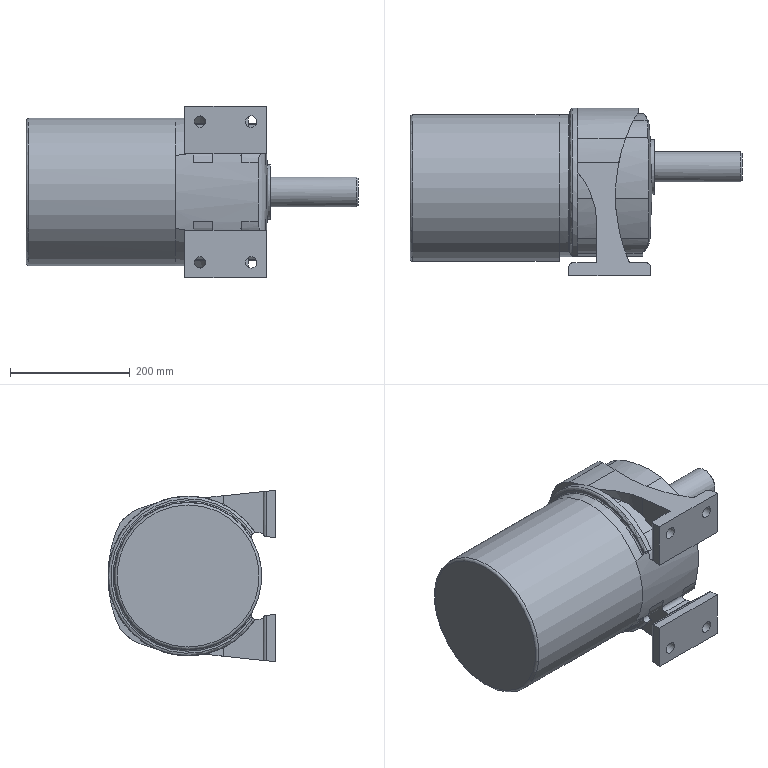Part | NX | features BREP 1 | 1 solid | 88 faces | box 553.467 x 279.469 x 285.867 mm | volume 20300035 mm3 | cylinder 48 | plane 31 | torus 5 | cone 3 | sphere 1 | commonest cylinder face diameters 12.8 x14 19.2 x4 106.667 x4 358.4 x4 494.933 x4 108.8 x2